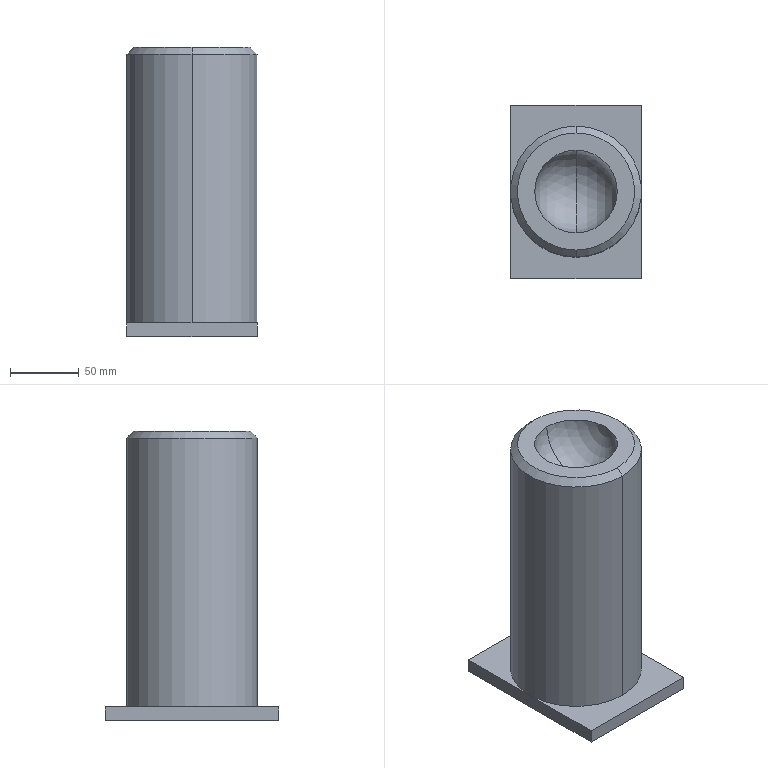Part | SolidWorks | features Extrusion 1, Revolution 1 | 2 solids | 14 faces | box 95 x 126 x 210 mm | volume 1477195 mm3 | plane 8 | sphere 2 | cone 2 | cylinder 2 | commonest cylinder face diameters 95 x2
STEP:
#1=CARTESIAN_POINT('',(47.5,-63.,0.));
#2=VERTEX_POINT('',#1);
#3=CARTESIAN_POINT('',(47.5,63.,0.));
#4=VERTEX_POINT('',#3);
#5=CARTESIAN_POINT('',(47.5,-63.,0.));
#6=DIRECTION('',(0.,1.,0.));
#7=VECTOR('',#6,1000.);
#8=LINE('',#5,#7);
#9=EDGE_CURVE('',#2,#4,#8,.T.);
#10=ORIENTED_EDGE('',*,*,#9,.T.);
#11=CARTESIAN_POINT('',(47.5,63.,10.));
#12=VERTEX_POINT('',#11);
#13=CARTESIAN_POINT('',(47.5,63.,10.));
#14=DIRECTION('',(0.,0.,-1.));
#15=VECTOR('',#14,1000.);
#16=LINE('',#13,#15);
#17=EDGE_CURVE('',#12,#4,#16,.T.);
#18=ORIENTED_EDGE('',*,*,#17,.F.);
#19=CARTESIAN_POINT('',(47.5,-63.,10.));
#20=VERTEX_POINT('',#19);
#21=CARTESIAN_POINT('',(47.5,-63.,10.));
#22=DIRECTION('',(0.,1.,0.));
#23=VECTOR('',#22,1000.);
#24=LINE('',#21,#23);
#25=EDGE_CURVE('',#20,#12,#24,.T.);
#26=ORIENTED_EDGE('',*,*,#25,.F.);
#27=CARTESIAN_POINT('',(47.5,-63.,10.));
#28=DIRECTION('',(0.,0.,-1.));
#29=VECTOR('',#28,1000.);
#30=LINE('',#27,#29);
#31=EDGE_CURVE('',#20,#2,#30,.T.);
#32=ORIENTED_EDGE('',*,*,#31,.T.);
#33=EDGE_LOOP('',(#10,#18,#26,#32));
#34=FACE_OUTER_BOUND('',#33,.T.);
#35=CARTESIAN_POINT('',(47.5,-63.,10.));
#36=DIRECTION('',(-1.,0.,0.));
#37=DIRECTION('',(0.,0.,1.));
#38=AXIS2_PLACEMENT_3D('',#35,#36,#37);
#39=PLANE('',#38);
#40=ADVANCED_FACE('',(#34),#39,.F.);
#41=CARTESIAN_POINT('',(-47.5,63.,0.));
#42=VERTEX_POINT('',#41);
#43=CARTESIAN_POINT('',(47.5,63.,0.));
#44=DIRECTION('',(-1.,0.,0.));
#45=VECTOR('',#44,1000.);
#46=LINE('',#43,#45);
#47=EDGE_CURVE('',#4,#42,#46,.T.);
#48=ORIENTED_EDGE('',*,*,#47,.T.);
#49=CARTESIAN_POINT('',(-47.5,63.,10.));
#50=VERTEX_POINT('',#49);
#51=CARTESIAN_POINT('',(-47.5,63.,10.));
#52=DIRECTION('',(0.,0.,-1.));
#53=VECTOR('',#52,1000.);
#54=LINE('',#51,#53);
#55=EDGE_CURVE('',#50,#42,#54,.T.);
#56=ORIENTED_EDGE('',*,*,#55,.F.);
#57=CARTESIAN_POINT('',(47.5,63.,10.));
#58=DIRECTION('',(-1.,0.,0.));
#59=VECTOR('',#58,1000.);
#60=LINE('',#57,#59);
#61=EDGE_CURVE('',#12,#50,#60,.T.);
#62=ORIENTED_EDGE('',*,*,#61,.F.);
#63=ORIENTED_EDGE('',*,*,#17,.T.);
#64=EDGE_LOOP('',(#48,#56,#62,#63));
#65=FACE_OUTER_BOUND('',#64,.T.);
#66=CARTESIAN_POINT('',(47.5,63.,10.));
#67=DIRECTION('',(0.,-1.,0.));
#68=DIRECTION('',(0.,0.,-1.));
#69=AXIS2_PLACEMENT_3D('',#66,#67,#68);
#70=PLANE('',#69);
#71=ADVANCED_FACE('',(#65),#70,.F.);
#72=CARTESIAN_POINT('',(-47.5,-63.,0.));
#73=VERTEX_POINT('',#72);
#74=CARTESIAN_POINT('',(-47.5,-63.,0.));
#75=DIRECTION('',(0.,-1.,0.));
#76=VECTOR('',#75,1000.);
#77=LINE('',#74,#76);
#78=EDGE_CURVE('',#42,#73,#77,.T.);
#79=ORIENTED_EDGE('',*,*,#78,.T.);
#80=CARTESIAN_POINT('',(-47.5,-63.,10.));
#81=VERTEX_POINT('',#80);
#82=CARTESIAN_POINT('',(-47.5,-63.,10.));
#83=DIRECTION('',(0.,0.,-1.));
#84=VECTOR('',#83,1000.);
#85=LINE('',#82,#84);
#86=EDGE_CURVE('',#81,#73,#85,.T.);
#87=ORIENTED_EDGE('',*,*,#86,.F.);
#88=CARTESIAN_POINT('',(-47.5,-63.,10.));
#89=DIRECTION('',(0.,-1.,0.));
#90=VECTOR('',#89,1000.);
#91=LINE('',#88,#90);
#92=EDGE_CURVE('',#50,#81,#91,.T.);
#93=ORIENTED_EDGE('',*,*,#92,.F.);
#94=ORIENTED_EDGE('',*,*,#55,.T.);
#95=EDGE_LOOP('',(#79,#87,#93,#94));
#96=FACE_OUTER_BOUND('',#95,.T.);
#97=CARTESIAN_POINT('',(-47.5,-63.,10.));
#98=DIRECTION('',(1.,0.,0.));
#99=DIRECTION('',(0.,0.,-1.));
#100=AXIS2_PLACEMENT_3D('',#97,#98,#99);
#101=PLANE('',#100);
#102=ADVANCED_FACE('',(#96),#101,.F.);
#103=CARTESIAN_POINT('',(47.5,-63.,0.));
#104=DIRECTION('',(1.,0.,0.));
#105=VECTOR('',#104,1000.);
#106=LINE('',#103,#105);
#107=EDGE_CURVE('',#73,#2,#106,.T.);
#108=ORIENTED_EDGE('',*,*,#107,.T.);
#109=ORIENTED_EDGE('',*,*,#31,.F.);
#110=CARTESIAN_POINT('',(47.5,-63.,10.));
#111=DIRECTION('',(1.,0.,0.));
#112=VECTOR('',#111,1000.);
#113=LINE('',#110,#112);
#114=EDGE_CURVE('',#81,#20,#113,.T.);
#115=ORIENTED_EDGE('',*,*,#114,.F.);
#116=ORIENTED_EDGE('',*,*,#86,.T.);
#117=EDGE_LOOP('',(#108,#109,#115,#116));
#118=FACE_OUTER_BOUND('',#117,.T.);
#119=CARTESIAN_POINT('',(47.5,-63.,10.));
#120=DIRECTION('',(0.,1.,0.));
#121=DIRECTION('',(0.,0.,1.));
#122=AXIS2_PLACEMENT_3D('',#119,#120,#121);
#123=PLANE('',#122);
#124=ADVANCED_FACE('',(#118),#123,.F.);
#125=ORIENTED_EDGE('',*,*,#25,.T.);
#126=ORIENTED_EDGE('',*,*,#61,.T.);
#127=ORIENTED_EDGE('',*,*,#92,.T.);
#128=ORIENTED_EDGE('',*,*,#114,.T.);
#129=EDGE_LOOP('',(#125,#126,#127,#128));
#130=FACE_OUTER_BOUND('',#129,.T.);
#131=CARTESIAN_POINT('',(47.5,63.,10.));
#132=DIRECTION('',(0.,0.,1.));
#133=DIRECTION('',(1.,0.,0.));
#134=AXIS2_PLACEMENT_3D('',#131,#132,#133);
#135=PLANE('',#134);
#136=ADVANCED_FACE('',(#130),#135,.T.);
#137=ORIENTED_EDGE('',*,*,#9,.F.);
#138=ORIENTED_EDGE('',*,*,#107,.F.);
#139=ORIENTED_EDGE('',*,*,#78,.F.);
#140=ORIENTED_EDGE('',*,*,#47,.F.);
#141=EDGE_LOOP('',(#137,#138,#139,#140));
#142=FACE_OUTER_BOUND('',#141,.T.);
#143=CARTESIAN_POINT('',(47.5,63.,0.));
#144=DIRECTION('',(0.,0.,1.));
#145=DIRECTION('',(1.,0.,0.));
#146=AXIS2_PLACEMENT_3D('',#143,#144,#145);
#147=PLANE('',#146);
#148=ADVANCED_FACE('',(#142),#147,.F.);
#149=CLOSED_SHELL('',(#40,#71,#102,#124,#136,#148));
#150=MANIFOLD_SOLID_BREP('',#149);
#151=CARTESIAN_POINT('',(0.,-30.,210.));
#152=VERTEX_POINT('',#151);
#153=CARTESIAN_POINT('',(0.,30.,210.));
#154=VERTEX_POINT('',#153);
#155=CARTESIAN_POINT('',(0.,0.,210.));
#156=DIRECTION('',(0.,0.,-1.));
#157=DIRECTION('',(0.,1.,0.));
#158=AXIS2_PLACEMENT_3D('',#155,#156,#157);
#159=CIRCLE('',#158,30.);
#160=EDGE_CURVE('',#152,#154,#159,.T.);
#161=ORIENTED_EDGE('',*,*,#160,.F.);
#162=CARTESIAN_POINT('',(0.,0.,180.));
#163=VERTEX_POINT('',#162);
#164=CARTESIAN_POINT('',(0.,0.,210.));
#165=DIRECTION('',(1.,0.,0.));
#166=DIRECTION('',(0.,1.,0.));
#167=AXIS2_PLACEMENT_3D('',#164,#165,#166);
#168=CIRCLE('',#167,30.);
#169=EDGE_CURVE('',#152,#163,#168,.T.);
#170=ORIENTED_EDGE('',*,*,#169,.T.);
#171=CARTESIAN_POINT('',(0.,0.,210.));
#172=DIRECTION('',(-1.,0.,0.));
#173=DIRECTION('',(0.,0.,1.));
#174=AXIS2_PLACEMENT_3D('',#171,#172,#173);
#175=CIRCLE('',#174,30.);
#176=EDGE_CURVE('',#154,#163,#175,.T.);
#177=ORIENTED_EDGE('',*,*,#176,.F.);
#178=EDGE_LOOP('',(#161,#170,#177));
#179=FACE_OUTER_BOUND('',#178,.T.);
#180=CARTESIAN_POINT('',(0.,0.,210.));
#181=DIRECTION('',(1.,0.,0.));
#182=DIRECTION('',(0.,1.,0.));
#183=AXIS2_PLACEMENT_3D('',#180,#181,#182);
#184=SPHERICAL_SURFACE('',#183,30.);
#185=ADVANCED_FACE('',(#179),#184,.F.);
#186=CARTESIAN_POINT('',(0.,42.5,210.));
#187=VERTEX_POINT('',#186);
#188=CARTESIAN_POINT('',(0.,-42.5,210.));
#189=VERTEX_POINT('',#188);
#190=CARTESIAN_POINT('',(0.,0.,210.));
#191=DIRECTION('',(0.,0.,-1.));
#192=DIRECTION('',(0.,1.,0.));
#193=AXIS2_PLACEMENT_3D('',#190,#191,#192);
#194=CIRCLE('',#193,42.5);
#195=EDGE_CURVE('',#187,#189,#194,.T.);
#196=ORIENTED_EDGE('',*,*,#195,.T.);
#197=CARTESIAN_POINT('',(0.,-47.5,205.));
#198=VERTEX_POINT('',#197);
#199=CARTESIAN_POINT('',(0.,-47.5,205.));
#200=DIRECTION('',(0.,-0.7071,-0.7071));
#201=VECTOR('',#200,1000.);
#202=LINE('',#199,#201);
#203=EDGE_CURVE('',#189,#198,#202,.T.);
#204=ORIENTED_EDGE('',*,*,#203,.T.);
#205=CARTESIAN_POINT('',(0.,47.5,205.));
#206=VERTEX_POINT('',#205);
#207=CARTESIAN_POINT('',(0.,0.,205.));
#208=DIRECTION('',(0.,0.,-1.));
#209=DIRECTION('',(0.,1.,0.));
#210=AXIS2_PLACEMENT_3D('',#207,#208,#209);
#211=CIRCLE('',#210,47.5);
#212=EDGE_CURVE('',#206,#198,#211,.T.);
#213=ORIENTED_EDGE('',*,*,#212,.F.);
#214=CARTESIAN_POINT('',(0.,47.5,205.));
#215=DIRECTION('',(0.,0.7071,-0.7071));
#216=VECTOR('',#215,1000.);
#217=LINE('',#214,#216);
#218=EDGE_CURVE('',#187,#206,#217,.T.);
#219=ORIENTED_EDGE('',*,*,#218,.F.);
#220=EDGE_LOOP('',(#196,#204,#213,#219));
#221=FACE_OUTER_BOUND('',#220,.T.);
#222=CARTESIAN_POINT('',(0.,0.,205.));
#223=DIRECTION('',(0.,0.,-1.));
#224=DIRECTION('',(0.,1.,0.));
#225=AXIS2_PLACEMENT_3D('',#222,#223,#224);
#226=CONICAL_SURFACE('',#225,47.5,0.7854);
#227=ADVANCED_FACE('',(#221),#226,.T.);
#228=ORIENTED_EDGE('',*,*,#212,.T.);
#229=CARTESIAN_POINT('',(0.,-47.5,10.));
#230=VERTEX_POINT('',#229);
#231=CARTESIAN_POINT('',(0.,-47.5,10.));
#232=DIRECTION('',(0.,0.,-1.));
#233=VECTOR('',#232,1000.);
#234=LINE('',#231,#233);
#235=EDGE_CURVE('',#198,#230,#234,.T.);
#236=ORIENTED_EDGE('',*,*,#235,.T.);
#237=CARTESIAN_POINT('',(0.,47.5,10.));
#238=VERTEX_POINT('',#237);
#239=CARTESIAN_POINT('',(0.,0.,10.));
#240=DIRECTION('',(0.,0.,-1.));
#241=DIRECTION('',(0.,1.,0.));
#242=AXIS2_PLACEMENT_3D('',#239,#240,#241);
#243=CIRCLE('',#242,47.5);
#244=EDGE_CURVE('',#238,#230,#243,.T.);
#245=ORIENTED_EDGE('',*,*,#244,.F.);
#246=CARTESIAN_POINT('',(0.,47.5,10.));
#247=DIRECTION('',(0.,0.,-1.));
#248=VECTOR('',#247,1000.);
#249=LINE('',#246,#248);
#250=EDGE_CURVE('',#206,#238,#249,.T.);
#251=ORIENTED_EDGE('',*,*,#250,.F.);
#252=EDGE_LOOP('',(#228,#236,#245,#251));
#253=FACE_OUTER_BOUND('',#252,.T.);
#254=CARTESIAN_POINT('',(0.,0.,10.));
#255=DIRECTION('',(0.,0.,-1.));
#256=DIRECTION('',(0.,1.,0.));
#257=AXIS2_PLACEMENT_3D('',#254,#255,#256);
#258=CYLINDRICAL_SURFACE('',#257,47.5);
#259=ADVANCED_FACE('',(#253),#258,.T.);
#260=ORIENTED_EDGE('',*,*,#244,.T.);
#261=CARTESIAN_POINT('',(0.,0.,10.));
#262=DIRECTION('',(0.,0.,-1.));
#263=DIRECTION('',(0.,1.,0.));
#264=AXIS2_PLACEMENT_3D('',#261,#262,#263);
#265=CIRCLE('',#264,47.5);
#266=EDGE_CURVE('',#230,#238,#265,.T.);
#267=ORIENTED_EDGE('',*,*,#266,.T.);
#268=EDGE_LOOP('',(#260,#267));
#269=FACE_OUTER_BOUND('',#268,.T.);
#270=CARTESIAN_POINT('',(0.,0.,10.));
#271=DIRECTION('',(0.,0.,-1.));
#272=DIRECTION('',(0.,1.,0.));
#273=AXIS2_PLACEMENT_3D('',#270,#271,#272);
#274=PLANE('',#273);
#275=ADVANCED_FACE('',(#269),#274,.T.);
#276=ORIENTED_EDGE('',*,*,#235,.F.);
#277=CARTESIAN_POINT('',(0.,0.,205.));
#278=DIRECTION('',(0.,0.,-1.));
#279=DIRECTION('',(0.,1.,0.));
#280=AXIS2_PLACEMENT_3D('',#277,#278,#279);
#281=CIRCLE('',#280,47.5);
#282=EDGE_CURVE('',#198,#206,#281,.T.);
#283=ORIENTED_EDGE('',*,*,#282,.T.);
#284=ORIENTED_EDGE('',*,*,#250,.T.);
#285=ORIENTED_EDGE('',*,*,#266,.F.);
#286=EDGE_LOOP('',(#276,#283,#284,#285));
#287=FACE_OUTER_BOUND('',#286,.T.);
#288=CARTESIAN_POINT('',(0.,0.,10.));
#289=DIRECTION('',(0.,0.,-1.));
#290=DIRECTION('',(0.,1.,0.));
#291=AXIS2_PLACEMENT_3D('',#288,#289,#290);
#292=CYLINDRICAL_SURFACE('',#291,47.5);
#293=ADVANCED_FACE('',(#287),#292,.T.);
#294=ORIENTED_EDGE('',*,*,#203,.F.);
#295=CARTESIAN_POINT('',(0.,0.,210.));
#296=DIRECTION('',(0.,0.,-1.));
#297=DIRECTION('',(0.,1.,0.));
#298=AXIS2_PLACEMENT_3D('',#295,#296,#297);
#299=CIRCLE('',#298,42.5);
#300=EDGE_CURVE('',#189,#187,#299,.T.);
#301=ORIENTED_EDGE('',*,*,#300,.T.);
#302=ORIENTED_EDGE('',*,*,#218,.T.);
#303=ORIENTED_EDGE('',*,*,#282,.F.);
#304=EDGE_LOOP('',(#294,#301,#302,#303));
#305=FACE_OUTER_BOUND('',#304,.T.);
#306=CARTESIAN_POINT('',(0.,0.,205.));
#307=DIRECTION('',(0.,0.,-1.));
#308=DIRECTION('',(0.,1.,0.));
#309=AXIS2_PLACEMENT_3D('',#306,#307,#308);
#310=CONICAL_SURFACE('',#309,47.5,0.7854);
#311=ADVANCED_FACE('',(#305),#310,.T.);
#312=CARTESIAN_POINT('',(0.,0.,210.));
#313=DIRECTION('',(0.,0.,-1.));
#314=DIRECTION('',(0.,1.,0.));
#315=AXIS2_PLACEMENT_3D('',#312,#313,#314);
#316=CIRCLE('',#315,30.);
#317=EDGE_CURVE('',#154,#152,#316,.T.);
#318=ORIENTED_EDGE('',*,*,#317,.T.);
#319=ORIENTED_EDGE('',*,*,#160,.T.);
#320=EDGE_LOOP('',(#318,#319));
#321=FACE_BOUND('',#320,.T.);
#322=ORIENTED_EDGE('',*,*,#195,.F.);
#323=ORIENTED_EDGE('',*,*,#300,.F.);
#324=EDGE_LOOP('',(#322,#323));
#325=FACE_OUTER_BOUND('',#324,.T.);
#326=CARTESIAN_POINT('',(0.,30.,210.));
#327=DIRECTION('',(0.,0.,1.));
#328=DIRECTION('',(0.,-1.,0.));
#329=AXIS2_PLACEMENT_3D('',#326,#327,#328);
#330=PLANE('',#329);
#331=ADVANCED_FACE('',(#321,#325),#330,.T.);
#332=ORIENTED_EDGE('',*,*,#169,.F.);
#333=ORIENTED_EDGE('',*,*,#317,.F.);
#334=ORIENTED_EDGE('',*,*,#176,.T.);
#335=EDGE_LOOP('',(#332,#333,#334));
#336=FACE_OUTER_BOUND('',#335,.T.);
#337=CARTESIAN_POINT('',(0.,0.,210.));
#338=DIRECTION('',(1.,0.,0.));
#339=DIRECTION('',(0.,1.,0.));
#340=AXIS2_PLACEMENT_3D('',#337,#338,#339);
#341=SPHERICAL_SURFACE('',#340,30.);
#342=ADVANCED_FACE('',(#336),#341,.F.);
#343=CLOSED_SHELL('',(#185,#227,#259,#275,#293,#311,#331,#342));
#344=MANIFOLD_SOLID_BREP('',#343);
#345=CARTESIAN_POINT('',(0.,0.,0.));
#346=DIRECTION('',(0.,0.,1.));
#347=DIRECTION('',(1.,0.,0.));
#348=AXIS2_PLACEMENT_3D('',#345,#346,#347);
#349=(LENGTH_UNIT()NAMED_UNIT(*)SI_UNIT(.MILLI.,.METRE.));
#350=UNCERTAINTY_MEASURE_WITH_UNIT(LENGTH_MEASURE(0.00001),#349,'','');
#351=(NAMED_UNIT(*)PLANE_ANGLE_UNIT()SI_UNIT($,.RADIAN.));
#352=(NAMED_UNIT(*)SI_UNIT($,.STERADIAN.)SOLID_ANGLE_UNIT());
#353=(GEOMETRIC_REPRESENTATION_CONTEXT(3)GLOBAL_UNCERTAINTY_ASSIGNED_CONTEXT((#350))GLOBAL_UNIT_ASSIGNED_CONTEXT((#349,#351,#352))REPRESENTATION_CONTEXT('',''));
#354=ADVANCED_BREP_SHAPE_REPRESENTATION('',(#150,#344,#348),#353);